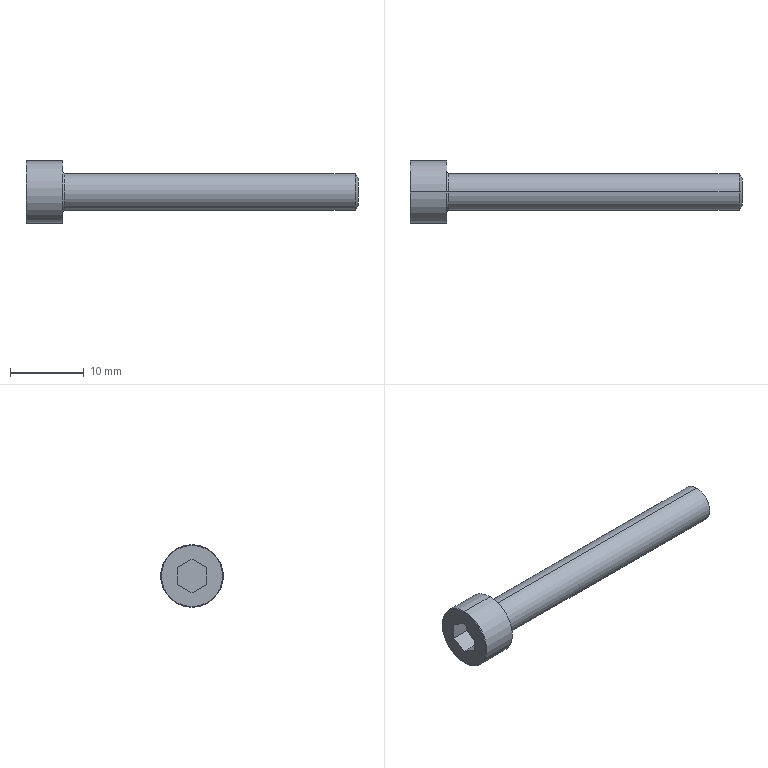Part | STEP file | 1 solid | 20 faces | box 45 x 8.5 x 8.5 mm | volume 1033 mm3 | plane 10 | torus 4 | cylinder 4 | cone 2 | commonest cylinder face diameters 5 x2 8.5 x2
STEP:
#1=CARTESIAN_POINT('',(0.,0.,4.15));
#2=VERTEX_POINT('',#1);
#3=CARTESIAN_POINT('',(0.,0.,-4.15));
#4=VERTEX_POINT('',#3);
#5=CARTESIAN_POINT('',(0.,0.,0.));
#6=DIRECTION('',(-1.,0.,0.));
#7=DIRECTION('',(0.,0.,-1.));
#8=AXIS2_PLACEMENT_3D('',#5,#6,#7);
#9=CIRCLE('',#8,4.15);
#10=EDGE_CURVE('',#2,#4,#9,.T.);
#11=ORIENTED_EDGE('',*,*,#10,.F.);
#12=CARTESIAN_POINT('',(0.1,0.,4.25));
#13=VERTEX_POINT('',#12);
#14=CARTESIAN_POINT('',(0.1,0.,4.15));
#15=DIRECTION('',(0.,1.,0.));
#16=DIRECTION('',(0.,0.,1.));
#17=AXIS2_PLACEMENT_3D('',#14,#15,#16);
#18=CIRCLE('',#17,0.1);
#19=EDGE_CURVE('',#2,#13,#18,.T.);
#20=ORIENTED_EDGE('',*,*,#19,.T.);
#21=CARTESIAN_POINT('',(0.1,0.,-4.25));
#22=VERTEX_POINT('',#21);
#23=CARTESIAN_POINT('',(0.1,0.,0.));
#24=DIRECTION('',(1.,0.,0.));
#25=DIRECTION('',(0.,0.,-1.));
#26=AXIS2_PLACEMENT_3D('',#23,#24,#25);
#27=CIRCLE('',#26,4.25);
#28=EDGE_CURVE('',#22,#13,#27,.T.);
#29=ORIENTED_EDGE('',*,*,#28,.F.);
#30=CARTESIAN_POINT('',(0.1,0.,-4.15));
#31=DIRECTION('',(0.,-1.,0.));
#32=DIRECTION('',(0.,0.,-1.));
#33=AXIS2_PLACEMENT_3D('',#30,#31,#32);
#34=CIRCLE('',#33,0.1);
#35=EDGE_CURVE('',#4,#22,#34,.T.);
#36=ORIENTED_EDGE('',*,*,#35,.F.);
#37=EDGE_LOOP('',(#11,#20,#29,#36));
#38=FACE_OUTER_BOUND('',#37,.T.);
#39=CARTESIAN_POINT('',(0.1,0.,0.));
#40=DIRECTION('',(1.,0.,0.));
#41=DIRECTION('',(0.,0.,-1.));
#42=AXIS2_PLACEMENT_3D('',#39,#40,#41);
#43=TOROIDAL_SURFACE('',#42,4.15,0.1);
#44=ADVANCED_FACE('',(#38),#43,.T.);
#45=CARTESIAN_POINT('',(45.,0.,1.807));
#46=VERTEX_POINT('',#45);
#47=CARTESIAN_POINT('',(45.,0.,-1.807));
#48=VERTEX_POINT('',#47);
#49=CARTESIAN_POINT('',(45.,0.,0.));
#50=DIRECTION('',(-1.,0.,0.));
#51=DIRECTION('',(0.,0.,1.));
#52=AXIS2_PLACEMENT_3D('',#49,#50,#51);
#53=CIRCLE('',#52,1.807);
#54=EDGE_CURVE('',#46,#48,#53,.T.);
#55=ORIENTED_EDGE('',*,*,#54,.T.);
#56=CARTESIAN_POINT('',(44.6,0.,-2.5));
#57=VERTEX_POINT('',#56);
#58=CARTESIAN_POINT('',(44.6,0.,-2.5));
#59=DIRECTION('',(-0.5,0.,-0.866));
#60=VECTOR('',#59,1000.);
#61=LINE('',#58,#60);
#62=EDGE_CURVE('',#48,#57,#61,.T.);
#63=ORIENTED_EDGE('',*,*,#62,.T.);
#64=CARTESIAN_POINT('',(44.6,0.,2.5));
#65=VERTEX_POINT('',#64);
#66=CARTESIAN_POINT('',(44.6,0.,0.));
#67=DIRECTION('',(-1.,0.,0.));
#68=DIRECTION('',(0.,0.,1.));
#69=AXIS2_PLACEMENT_3D('',#66,#67,#68);
#70=CIRCLE('',#69,2.5);
#71=EDGE_CURVE('',#65,#57,#70,.T.);
#72=ORIENTED_EDGE('',*,*,#71,.F.);
#73=CARTESIAN_POINT('',(44.6,0.,2.5));
#74=DIRECTION('',(-0.5,0.,0.866));
#75=VECTOR('',#74,1000.);
#76=LINE('',#73,#75);
#77=EDGE_CURVE('',#46,#65,#76,.T.);
#78=ORIENTED_EDGE('',*,*,#77,.F.);
#79=EDGE_LOOP('',(#55,#63,#72,#78));
#80=FACE_OUTER_BOUND('',#79,.T.);
#81=CARTESIAN_POINT('',(44.6,0.,0.));
#82=DIRECTION('',(-1.,0.,0.));
#83=DIRECTION('',(0.,0.,1.));
#84=AXIS2_PLACEMENT_3D('',#81,#82,#83);
#85=CONICAL_SURFACE('',#84,2.5,1.047);
#86=ADVANCED_FACE('',(#80),#85,.T.);
#87=CARTESIAN_POINT('',(5.,0.,-2.7));
#88=VERTEX_POINT('',#87);
#89=CARTESIAN_POINT('',(5.,0.,2.7));
#90=VERTEX_POINT('',#89);
#91=CARTESIAN_POINT('',(5.,0.,0.));
#92=DIRECTION('',(-1.,0.,0.));
#93=DIRECTION('',(0.,0.,1.));
#94=AXIS2_PLACEMENT_3D('',#91,#92,#93);
#95=CIRCLE('',#94,2.7);
#96=EDGE_CURVE('',#88,#90,#95,.T.);
#97=ORIENTED_EDGE('',*,*,#96,.F.);
#98=CARTESIAN_POINT('',(5.2,0.,-2.5));
#99=VERTEX_POINT('',#98);
#100=CARTESIAN_POINT('',(5.2,0.,-2.7));
#101=DIRECTION('',(0.,1.,0.));
#102=DIRECTION('',(0.,0.,1.));
#103=AXIS2_PLACEMENT_3D('',#100,#101,#102);
#104=CIRCLE('',#103,0.2);
#105=EDGE_CURVE('',#88,#99,#104,.T.);
#106=ORIENTED_EDGE('',*,*,#105,.T.);
#107=CARTESIAN_POINT('',(5.2,0.,2.5));
#108=VERTEX_POINT('',#107);
#109=CARTESIAN_POINT('',(5.2,0.,0.));
#110=DIRECTION('',(-1.,0.,0.));
#111=DIRECTION('',(0.,0.,1.));
#112=AXIS2_PLACEMENT_3D('',#109,#110,#111);
#113=CIRCLE('',#112,2.5);
#114=EDGE_CURVE('',#99,#108,#113,.T.);
#115=ORIENTED_EDGE('',*,*,#114,.T.);
#116=CARTESIAN_POINT('',(5.2,0.,2.7));
#117=DIRECTION('',(0.,-1.,0.));
#118=DIRECTION('',(0.,0.,-1.));
#119=AXIS2_PLACEMENT_3D('',#116,#117,#118);
#120=CIRCLE('',#119,0.2);
#121=EDGE_CURVE('',#90,#108,#120,.T.);
#122=ORIENTED_EDGE('',*,*,#121,.F.);
#123=EDGE_LOOP('',(#97,#106,#115,#122));
#124=FACE_OUTER_BOUND('',#123,.T.);
#125=CARTESIAN_POINT('',(5.2,0.,0.));
#126=DIRECTION('',(-1.,0.,0.));
#127=DIRECTION('',(0.,0.,1.));
#128=AXIS2_PLACEMENT_3D('',#125,#126,#127);
#129=TOROIDAL_SURFACE('',#128,2.7,0.2);
#130=ADVANCED_FACE('',(#124),#129,.F.);
#131=CARTESIAN_POINT('',(5.,0.,4.25));
#132=VERTEX_POINT('',#131);
#133=CARTESIAN_POINT('',(5.,0.,-4.25));
#134=VERTEX_POINT('',#133);
#135=CARTESIAN_POINT('',(5.,0.,0.));
#136=DIRECTION('',(-1.,0.,0.));
#137=DIRECTION('',(0.,0.,1.));
#138=AXIS2_PLACEMENT_3D('',#135,#136,#137);
#139=CIRCLE('',#138,4.25);
#140=EDGE_CURVE('',#132,#134,#139,.T.);
#141=ORIENTED_EDGE('',*,*,#140,.T.);
#142=CARTESIAN_POINT('',(0.,0.,-4.25));
#143=DIRECTION('',(-1.,0.,0.));
#144=VECTOR('',#143,1000.);
#145=LINE('',#142,#144);
#146=EDGE_CURVE('',#134,#22,#145,.T.);
#147=ORIENTED_EDGE('',*,*,#146,.T.);
#148=ORIENTED_EDGE('',*,*,#28,.T.);
#149=CARTESIAN_POINT('',(0.,0.,4.25));
#150=DIRECTION('',(-1.,0.,0.));
#151=VECTOR('',#150,1000.);
#152=LINE('',#149,#151);
#153=EDGE_CURVE('',#132,#13,#152,.T.);
#154=ORIENTED_EDGE('',*,*,#153,.F.);
#155=EDGE_LOOP('',(#141,#147,#148,#154));
#156=FACE_OUTER_BOUND('',#155,.T.);
#157=CARTESIAN_POINT('',(0.,0.,0.));
#158=DIRECTION('',(-1.,0.,0.));
#159=DIRECTION('',(0.,0.,1.));
#160=AXIS2_PLACEMENT_3D('',#157,#158,#159);
#161=CYLINDRICAL_SURFACE('',#160,4.25);
#162=ADVANCED_FACE('',(#156),#161,.T.);
#163=ORIENTED_EDGE('',*,*,#71,.T.);
#164=CARTESIAN_POINT('',(0.,0.,-2.5));
#165=DIRECTION('',(-1.,0.,0.));
#166=VECTOR('',#165,1000.);
#167=LINE('',#164,#166);
#168=EDGE_CURVE('',#57,#99,#167,.T.);
#169=ORIENTED_EDGE('',*,*,#168,.T.);
#170=CARTESIAN_POINT('',(5.2,0.,0.));
#171=DIRECTION('',(-1.,0.,0.));
#172=DIRECTION('',(0.,0.,1.));
#173=AXIS2_PLACEMENT_3D('',#170,#171,#172);
#174=CIRCLE('',#173,2.5);
#175=EDGE_CURVE('',#108,#99,#174,.T.);
#176=ORIENTED_EDGE('',*,*,#175,.F.);
#177=CARTESIAN_POINT('',(0.,0.,2.5));
#178=DIRECTION('',(-1.,0.,0.));
#179=VECTOR('',#178,1000.);
#180=LINE('',#177,#179);
#181=EDGE_CURVE('',#65,#108,#180,.T.);
#182=ORIENTED_EDGE('',*,*,#181,.F.);
#183=EDGE_LOOP('',(#163,#169,#176,#182));
#184=FACE_OUTER_BOUND('',#183,.T.);
#185=CARTESIAN_POINT('',(0.,0.,0.));
#186=DIRECTION('',(-1.,0.,0.));
#187=DIRECTION('',(0.,0.,1.));
#188=AXIS2_PLACEMENT_3D('',#185,#186,#187);
#189=CYLINDRICAL_SURFACE('',#188,2.5);
#190=ADVANCED_FACE('',(#184),#189,.T.);
#191=ORIENTED_EDGE('',*,*,#168,.F.);
#192=CARTESIAN_POINT('',(44.6,0.,0.));
#193=DIRECTION('',(-1.,0.,0.));
#194=DIRECTION('',(0.,0.,1.));
#195=AXIS2_PLACEMENT_3D('',#192,#193,#194);
#196=CIRCLE('',#195,2.5);
#197=EDGE_CURVE('',#57,#65,#196,.T.);
#198=ORIENTED_EDGE('',*,*,#197,.T.);
#199=ORIENTED_EDGE('',*,*,#181,.T.);
#200=ORIENTED_EDGE('',*,*,#114,.F.);
#201=EDGE_LOOP('',(#191,#198,#199,#200));
#202=FACE_OUTER_BOUND('',#201,.T.);
#203=CARTESIAN_POINT('',(0.,0.,0.));
#204=DIRECTION('',(-1.,0.,0.));
#205=DIRECTION('',(0.,0.,1.));
#206=AXIS2_PLACEMENT_3D('',#203,#204,#205);
#207=CYLINDRICAL_SURFACE('',#206,2.5);
#208=ADVANCED_FACE('',(#202),#207,.T.);
#209=CARTESIAN_POINT('',(0.,0.,0.));
#210=DIRECTION('',(-1.,0.,0.));
#211=DIRECTION('',(0.,0.,-1.));
#212=AXIS2_PLACEMENT_3D('',#209,#210,#211);
#213=CIRCLE('',#212,4.15);
#214=EDGE_CURVE('',#4,#2,#213,.T.);
#215=ORIENTED_EDGE('',*,*,#214,.T.);
#216=ORIENTED_EDGE('',*,*,#10,.T.);
#217=EDGE_LOOP('',(#215,#216));
#218=FACE_OUTER_BOUND('',#217,.T.);
#219=CARTESIAN_POINT('',(0.,0.,2.29));
#220=VERTEX_POINT('',#219);
#221=CARTESIAN_POINT('',(0.,1.983,1.145));
#222=VERTEX_POINT('',#221);
#223=CARTESIAN_POINT('',(0.,0.,2.29));
#224=DIRECTION('',(0.,0.866,-0.5));
#225=VECTOR('',#224,1000.);
#226=LINE('',#223,#225);
#227=EDGE_CURVE('',#220,#222,#226,.T.);
#228=ORIENTED_EDGE('',*,*,#227,.F.);
#229=CARTESIAN_POINT('',(0.,-1.983,1.145));
#230=VERTEX_POINT('',#229);
#231=CARTESIAN_POINT('',(0.,-1.983,1.145));
#232=DIRECTION('',(0.,0.866,0.5));
#233=VECTOR('',#232,1000.);
#234=LINE('',#231,#233);
#235=EDGE_CURVE('',#230,#220,#234,.T.);
#236=ORIENTED_EDGE('',*,*,#235,.F.);
#237=CARTESIAN_POINT('',(0.,-1.983,-1.145));
#238=VERTEX_POINT('',#237);
#239=CARTESIAN_POINT('',(0.,-1.983,-1.145));
#240=DIRECTION('',(0.,0.,1.));
#241=VECTOR('',#240,1000.);
#242=LINE('',#239,#241);
#243=EDGE_CURVE('',#238,#230,#242,.T.);
#244=ORIENTED_EDGE('',*,*,#243,.F.);
#245=CARTESIAN_POINT('',(0.,0.,-2.29));
#246=VERTEX_POINT('',#245);
#247=CARTESIAN_POINT('',(0.,0.,-2.29));
#248=DIRECTION('',(0.,-0.866,0.5));
#249=VECTOR('',#248,1000.);
#250=LINE('',#247,#249);
#251=EDGE_CURVE('',#246,#238,#250,.T.);
#252=ORIENTED_EDGE('',*,*,#251,.F.);
#253=CARTESIAN_POINT('',(0.,1.983,-1.145));
#254=VERTEX_POINT('',#253);
#255=CARTESIAN_POINT('',(0.,1.983,-1.145));
#256=DIRECTION('',(0.,-0.866,-0.5));
#257=VECTOR('',#256,1000.);
#258=LINE('',#255,#257);
#259=EDGE_CURVE('',#254,#246,#258,.T.);
#260=ORIENTED_EDGE('',*,*,#259,.F.);
#261=CARTESIAN_POINT('',(0.,1.983,1.145));
#262=DIRECTION('',(0.,0.,-1.));
#263=VECTOR('',#262,1000.);
#264=LINE('',#261,#263);
#265=EDGE_CURVE('',#222,#254,#264,.T.);
#266=ORIENTED_EDGE('',*,*,#265,.F.);
#267=EDGE_LOOP('',(#228,#236,#244,#252,#260,#266));
#268=FACE_BOUND('',#267,.T.);
#269=CARTESIAN_POINT('',(0.,0.,0.));
#270=DIRECTION('',(1.,0.,0.));
#271=DIRECTION('',(0.,0.,-1.));
#272=AXIS2_PLACEMENT_3D('',#269,#270,#271);
#273=PLANE('',#272);
#274=ADVANCED_FACE('',(#218,#268),#273,.F.);
#275=ORIENTED_EDGE('',*,*,#146,.F.);
#276=CARTESIAN_POINT('',(5.,0.,0.));
#277=DIRECTION('',(-1.,0.,0.));
#278=DIRECTION('',(0.,0.,1.));
#279=AXIS2_PLACEMENT_3D('',#276,#277,#278);
#280=CIRCLE('',#279,4.25);
#281=EDGE_CURVE('',#134,#132,#280,.T.);
#282=ORIENTED_EDGE('',*,*,#281,.T.);
#283=ORIENTED_EDGE('',*,*,#153,.T.);
#284=CARTESIAN_POINT('',(0.1,0.,0.));
#285=DIRECTION('',(1.,0.,0.));
#286=DIRECTION('',(0.,0.,-1.));
#287=AXIS2_PLACEMENT_3D('',#284,#285,#286);
#288=CIRCLE('',#287,4.25);
#289=EDGE_CURVE('',#13,#22,#288,.T.);
#290=ORIENTED_EDGE('',*,*,#289,.T.);
#291=EDGE_LOOP('',(#275,#282,#283,#290));
#292=FACE_OUTER_BOUND('',#291,.T.);
#293=CARTESIAN_POINT('',(0.,0.,0.));
#294=DIRECTION('',(-1.,0.,0.));
#295=DIRECTION('',(0.,0.,1.));
#296=AXIS2_PLACEMENT_3D('',#293,#294,#295);
#297=CYLINDRICAL_SURFACE('',#296,4.25);
#298=ADVANCED_FACE('',(#292),#297,.T.);
#299=ORIENTED_EDGE('',*,*,#140,.F.);
#300=ORIENTED_EDGE('',*,*,#281,.F.);
#301=EDGE_LOOP('',(#299,#300));
#302=FACE_OUTER_BOUND('',#301,.T.);
#303=CARTESIAN_POINT('',(5.,0.,0.));
#304=DIRECTION('',(-1.,0.,0.));
#305=DIRECTION('',(0.,0.,1.));
#306=AXIS2_PLACEMENT_3D('',#303,#304,#305);
#307=CIRCLE('',#306,2.7);
#308=EDGE_CURVE('',#90,#88,#307,.T.);
#309=ORIENTED_EDGE('',*,*,#308,.T.);
#310=ORIENTED_EDGE('',*,*,#96,.T.);
#311=EDGE_LOOP('',(#309,#310));
#312=FACE_BOUND('',#311,.T.);
#313=CARTESIAN_POINT('',(5.,4.25,0.));
#314=DIRECTION('',(-1.,0.,0.));
#315=DIRECTION('',(0.,0.,1.));
#316=AXIS2_PLACEMENT_3D('',#313,#314,#315);
#317=PLANE('',#316);
#318=ADVANCED_FACE('',(#302,#312),#317,.F.);
#319=ORIENTED_EDGE('',*,*,#105,.F.);
#320=ORIENTED_EDGE('',*,*,#308,.F.);
#321=ORIENTED_EDGE('',*,*,#121,.T.);
#322=ORIENTED_EDGE('',*,*,#175,.T.);
#323=EDGE_LOOP('',(#319,#320,#321,#322));
#324=FACE_OUTER_BOUND('',#323,.T.);
#325=CARTESIAN_POINT('',(5.2,0.,0.));
#326=DIRECTION('',(-1.,0.,0.));
#327=DIRECTION('',(0.,0.,1.));
#328=AXIS2_PLACEMENT_3D('',#325,#326,#327);
#329=TOROIDAL_SURFACE('',#328,2.7,0.2);
#330=ADVANCED_FACE('',(#324),#329,.F.);
#331=ORIENTED_EDGE('',*,*,#235,.T.);
#332=CARTESIAN_POINT('',(2.5,0.,2.29));
#333=VERTEX_POINT('',#332);
#334=CARTESIAN_POINT('',(2.5,0.,2.29));
#335=DIRECTION('',(-1.,0.,0.));
#336=VECTOR('',#335,1000.);
#337=LINE('',#334,#336);
#338=EDGE_CURVE('',#333,#220,#337,.T.);
#339=ORIENTED_EDGE('',*,*,#338,.F.);
#340=CARTESIAN_POINT('',(2.5,-1.983,1.145));
#341=VERTEX_POINT('',#340);
#342=CARTESIAN_POINT('',(2.5,-1.983,1.145));
#343=DIRECTION('',(0.,0.866,0.5));
#344=VECTOR('',#343,1000.);
#345=LINE('',#342,#344);
#346=EDGE_CURVE('',#341,#333,#345,.T.);
#347=ORIENTED_EDGE('',*,*,#346,.F.);
#348=CARTESIAN_POINT('',(2.5,-1.983,1.145));
#349=DIRECTION('',(-1.,0.,0.));
#350=VECTOR('',#349,1000.);
#351=LINE('',#348,#350);
#352=EDGE_CURVE('',#341,#230,#351,.T.);
#353=ORIENTED_EDGE('',*,*,#352,.T.);
#354=EDGE_LOOP('',(#331,#339,#347,#353));
#355=FACE_OUTER_BOUND('',#354,.T.);
#356=CARTESIAN_POINT('',(2.5,-1.983,1.145));
#357=DIRECTION('',(0.,-0.5,0.866));
#358=DIRECTION('',(0.,-0.866,-0.5));
#359=AXIS2_PLACEMENT_3D('',#356,#357,#358);
#360=PLANE('',#359);
#361=ADVANCED_FACE('',(#355),#360,.F.);
#362=ORIENTED_EDGE('',*,*,#243,.T.);
#363=ORIENTED_EDGE('',*,*,#352,.F.);
#364=CARTESIAN_POINT('',(2.5,-1.983,-1.145));
#365=VERTEX_POINT('',#364);
#366=CARTESIAN_POINT('',(2.5,-1.983,-1.145));
#367=DIRECTION('',(0.,0.,1.));
#368=VECTOR('',#367,1000.);
#369=LINE('',#366,#368);
#370=EDGE_CURVE('',#365,#341,#369,.T.);
#371=ORIENTED_EDGE('',*,*,#370,.F.);
#372=CARTESIAN_POINT('',(2.5,-1.983,-1.145));
#373=DIRECTION('',(-1.,0.,0.));
#374=VECTOR('',#373,1000.);
#375=LINE('',#372,#374);
#376=EDGE_CURVE('',#365,#238,#375,.T.);
#377=ORIENTED_EDGE('',*,*,#376,.T.);
#378=EDGE_LOOP('',(#362,#363,#371,#377));
#379=FACE_OUTER_BOUND('',#378,.T.);
#380=CARTESIAN_POINT('',(2.5,-1.983,-1.145));
#381=DIRECTION('',(0.,-1.,0.));
#382=DIRECTION('',(0.,0.,-1.));
#383=AXIS2_PLACEMENT_3D('',#380,#381,#382);
#384=PLANE('',#383);
#385=ADVANCED_FACE('',(#379),#384,.F.);
#386=ORIENTED_EDGE('',*,*,#251,.T.);
#387=ORIENTED_EDGE('',*,*,#376,.F.);
#388=CARTESIAN_POINT('',(2.5,0.,-2.29));
#389=VERTEX_POINT('',#388);
#390=CARTESIAN_POINT('',(2.5,0.,-2.29));
#391=DIRECTION('',(0.,-0.866,0.5));
#392=VECTOR('',#391,1000.);
#393=LINE('',#390,#392);
#394=EDGE_CURVE('',#389,#365,#393,.T.);
#395=ORIENTED_EDGE('',*,*,#394,.F.);
#396=CARTESIAN_POINT('',(2.5,0.,-2.29));
#397=DIRECTION('',(-1.,0.,0.));
#398=VECTOR('',#397,1000.);
#399=LINE('',#396,#398);
#400=EDGE_CURVE('',#389,#246,#399,.T.);
#401=ORIENTED_EDGE('',*,*,#400,.T.);
#402=EDGE_LOOP('',(#386,#387,#395,#401));
#403=FACE_OUTER_BOUND('',#402,.T.);
#404=CARTESIAN_POINT('',(2.5,0.,-2.29));
#405=DIRECTION('',(0.,-0.5,-0.866));
#406=DIRECTION('',(0.,0.866,-0.5));
#407=AXIS2_PLACEMENT_3D('',#404,#405,#406);
#408=PLANE('',#407);
#409=ADVANCED_FACE('',(#403),#408,.F.);
#410=ORIENTED_EDGE('',*,*,#259,.T.);
#411=ORIENTED_EDGE('',*,*,#400,.F.);
#412=CARTESIAN_POINT('',(2.5,1.983,-1.145));
#413=VERTEX_POINT('',#412);
#414=CARTESIAN_POINT('',(2.5,1.983,-1.145));
#415=DIRECTION('',(0.,-0.866,-0.5));
#416=VECTOR('',#415,1000.);
#417=LINE('',#414,#416);
#418=EDGE_CURVE('',#413,#389,#417,.T.);
#419=ORIENTED_EDGE('',*,*,#418,.F.);
#420=CARTESIAN_POINT('',(2.5,1.983,-1.145));
#421=DIRECTION('',(-1.,0.,0.));
#422=VECTOR('',#421,1000.);
#423=LINE('',#420,#422);
#424=EDGE_CURVE('',#413,#254,#423,.T.);
#425=ORIENTED_EDGE('',*,*,#424,.T.);
#426=EDGE_LOOP('',(#410,#411,#419,#425));
#427=FACE_OUTER_BOUND('',#426,.T.);
#428=CARTESIAN_POINT('',(2.5,1.983,-1.145));
#429=DIRECTION('',(0.,0.5,-0.866));
#430=DIRECTION('',(0.,0.866,0.5));
#431=AXIS2_PLACEMENT_3D('',#428,#429,#430);
#432=PLANE('',#431);
#433=ADVANCED_FACE('',(#427),#432,.F.);
#434=ORIENTED_EDGE('',*,*,#265,.T.);
#435=ORIENTED_EDGE('',*,*,#424,.F.);
#436=CARTESIAN_POINT('',(2.5,1.983,1.145));
#437=VERTEX_POINT('',#436);
#438=CARTESIAN_POINT('',(2.5,1.983,1.145));
#439=DIRECTION('',(0.,0.,-1.));
#440=VECTOR('',#439,1000.);
#441=LINE('',#438,#440);
#442=EDGE_CURVE('',#437,#413,#441,.T.);
#443=ORIENTED_EDGE('',*,*,#442,.F.);
#444=CARTESIAN_POINT('',(2.5,1.983,1.145));
#445=DIRECTION('',(-1.,0.,0.));
#446=VECTOR('',#445,1000.);
#447=LINE('',#444,#446);
#448=EDGE_CURVE('',#437,#222,#447,.T.);
#449=ORIENTED_EDGE('',*,*,#448,.T.);
#450=EDGE_LOOP('',(#434,#435,#443,#449));
#451=FACE_OUTER_BOUND('',#450,.T.);
#452=CARTESIAN_POINT('',(2.5,1.983,1.145));
#453=DIRECTION('',(0.,1.,0.));
#454=DIRECTION('',(0.,0.,1.));
#455=AXIS2_PLACEMENT_3D('',#452,#453,#454);
#456=PLANE('',#455);
#457=ADVANCED_FACE('',(#451),#456,.F.);
#458=ORIENTED_EDGE('',*,*,#227,.T.);
#459=ORIENTED_EDGE('',*,*,#448,.F.);
#460=CARTESIAN_POINT('',(2.5,0.,2.29));
#461=DIRECTION('',(0.,0.866,-0.5));
#462=VECTOR('',#461,1000.);
#463=LINE('',#460,#462);
#464=EDGE_CURVE('',#333,#437,#463,.T.);
#465=ORIENTED_EDGE('',*,*,#464,.F.);
#466=ORIENTED_EDGE('',*,*,#338,.T.);
#467=EDGE_LOOP('',(#458,#459,#465,#466));
#468=FACE_OUTER_BOUND('',#467,.T.);
#469=CARTESIAN_POINT('',(2.5,0.,2.29));
#470=DIRECTION('',(0.,0.5,0.866));
#471=DIRECTION('',(0.,-0.866,0.5));
#472=AXIS2_PLACEMENT_3D('',#469,#470,#471);
#473=PLANE('',#472);
#474=ADVANCED_FACE('',(#468),#473,.F.);
#475=ORIENTED_EDGE('',*,*,#346,.T.);
#476=ORIENTED_EDGE('',*,*,#464,.T.);
#477=ORIENTED_EDGE('',*,*,#442,.T.);
#478=ORIENTED_EDGE('',*,*,#418,.T.);
#479=ORIENTED_EDGE('',*,*,#394,.T.);
#480=ORIENTED_EDGE('',*,*,#370,.T.);
#481=EDGE_LOOP('',(#475,#476,#477,#478,#479,#480));
#482=FACE_OUTER_BOUND('',#481,.T.);
#483=CARTESIAN_POINT('',(2.5,-1.983,1.145));
#484=DIRECTION('',(1.,0.,0.));
#485=DIRECTION('',(0.,0.,-1.));
#486=AXIS2_PLACEMENT_3D('',#483,#484,#485);
#487=PLANE('',#486);
#488=ADVANCED_FACE('',(#482),#487,.F.);
#489=ORIENTED_EDGE('',*,*,#62,.F.);
#490=CARTESIAN_POINT('',(45.,0.,0.));
#491=DIRECTION('',(-1.,0.,0.));
#492=DIRECTION('',(0.,0.,1.));
#493=AXIS2_PLACEMENT_3D('',#490,#491,#492);
#494=CIRCLE('',#493,1.807);
#495=EDGE_CURVE('',#48,#46,#494,.T.);
#496=ORIENTED_EDGE('',*,*,#495,.T.);
#497=ORIENTED_EDGE('',*,*,#77,.T.);
#498=ORIENTED_EDGE('',*,*,#197,.F.);
#499=EDGE_LOOP('',(#489,#496,#497,#498));
#500=FACE_OUTER_BOUND('',#499,.T.);
#501=CARTESIAN_POINT('',(44.6,0.,0.));
#502=DIRECTION('',(-1.,0.,0.));
#503=DIRECTION('',(0.,0.,1.));
#504=AXIS2_PLACEMENT_3D('',#501,#502,#503);
#505=CONICAL_SURFACE('',#504,2.5,1.047);
#506=ADVANCED_FACE('',(#500),#505,.T.);
#507=ORIENTED_EDGE('',*,*,#54,.F.);
#508=ORIENTED_EDGE('',*,*,#495,.F.);
#509=EDGE_LOOP('',(#507,#508));
#510=FACE_OUTER_BOUND('',#509,.T.);
#511=CARTESIAN_POINT('',(45.,2.5,0.));
#512=DIRECTION('',(-1.,0.,0.));
#513=DIRECTION('',(0.,0.,1.));
#514=AXIS2_PLACEMENT_3D('',#511,#512,#513);
#515=PLANE('',#514);
#516=ADVANCED_FACE('',(#510),#515,.F.);
#517=ORIENTED_EDGE('',*,*,#19,.F.);
#518=ORIENTED_EDGE('',*,*,#214,.F.);
#519=ORIENTED_EDGE('',*,*,#35,.T.);
#520=ORIENTED_EDGE('',*,*,#289,.F.);
#521=EDGE_LOOP('',(#517,#518,#519,#520));
#522=FACE_OUTER_BOUND('',#521,.T.);
#523=CARTESIAN_POINT('',(0.1,0.,0.));
#524=DIRECTION('',(1.,0.,0.));
#525=DIRECTION('',(0.,0.,-1.));
#526=AXIS2_PLACEMENT_3D('',#523,#524,#525);
#527=TOROIDAL_SURFACE('',#526,4.15,0.1);
#528=ADVANCED_FACE('',(#522),#527,.T.);
#529=CLOSED_SHELL('',(#44,#86,#130,#162,#190,#208,#274,#298,#318,#330,#361,#385,#409,#433,#457,#474,#488,#506,#516,#528));
#530=MANIFOLD_SOLID_BREP('',#529);
#531=CARTESIAN_POINT('',(0.,0.,0.));
#532=DIRECTION('',(0.,0.,1.));
#533=DIRECTION('',(1.,0.,0.));
#534=AXIS2_PLACEMENT_3D('',#531,#532,#533);
#535=(LENGTH_UNIT()NAMED_UNIT(*)SI_UNIT(.MILLI.,.METRE.));
#536=UNCERTAINTY_MEASURE_WITH_UNIT(LENGTH_MEASURE(0.00001),#535,'','');
#537=(NAMED_UNIT(*)PLANE_ANGLE_UNIT()SI_UNIT($,.RADIAN.));
#538=(NAMED_UNIT(*)SI_UNIT($,.STERADIAN.)SOLID_ANGLE_UNIT());
#539=(GEOMETRIC_REPRESENTATION_CONTEXT(3)GLOBAL_UNCERTAINTY_ASSIGNED_CONTEXT((#536))GLOBAL_UNIT_ASSIGNED_CONTEXT((#535,#537,#538))REPRESENTATION_CONTEXT('',''));
#540=ADVANCED_BREP_SHAPE_REPRESENTATION('',(#530,#534),#539);